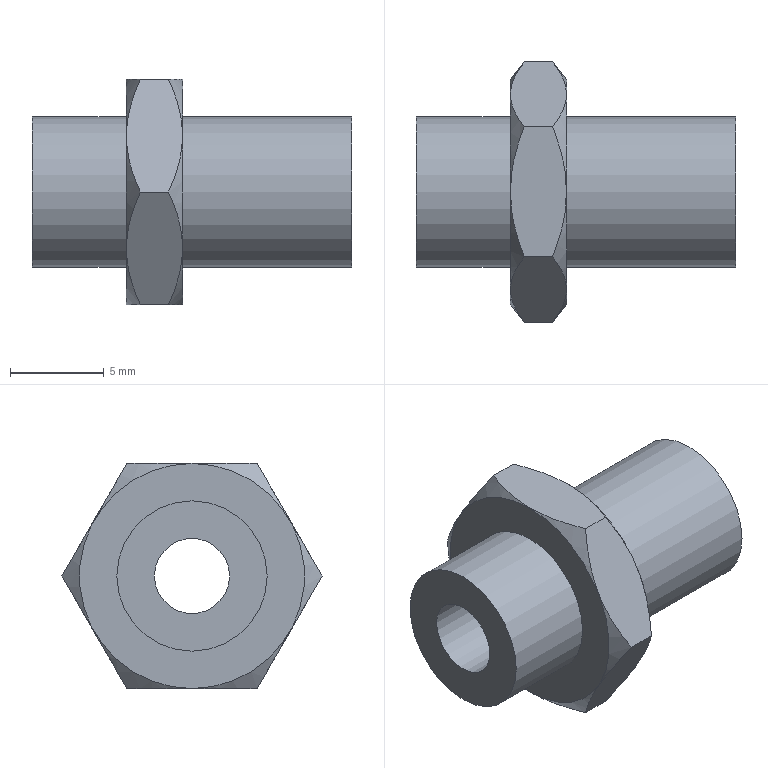Part | STEP file | 1-75.4 | 1 solid | 15 faces | box 17 x 13.856 x 12 mm | volume 858.508 mm3 | plane 10 | cylinder 3 | cone 2 | commonest cylinder face diameters 8 x2 4 x1